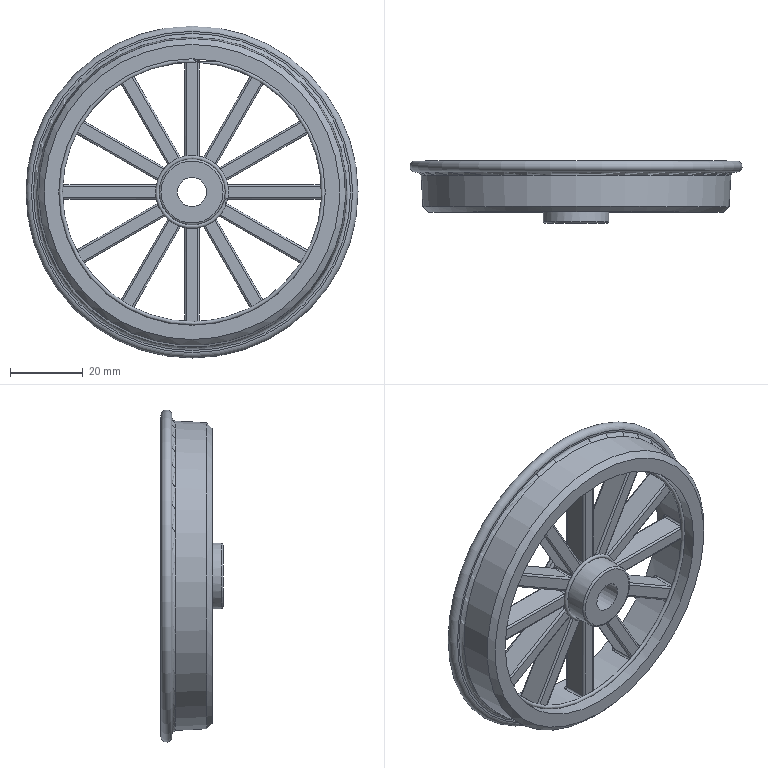Part | STEP file | 2-13.1 | 1 solid | 307 faces | box 91 x 17 x 91 mm | volume 34927 mm3 | cylinder 100 | spline 96 | torus 56 | plane 53 | cone 2 | commonest cylinder face diameters 1 x96 18 x2 8 x1 73 x1